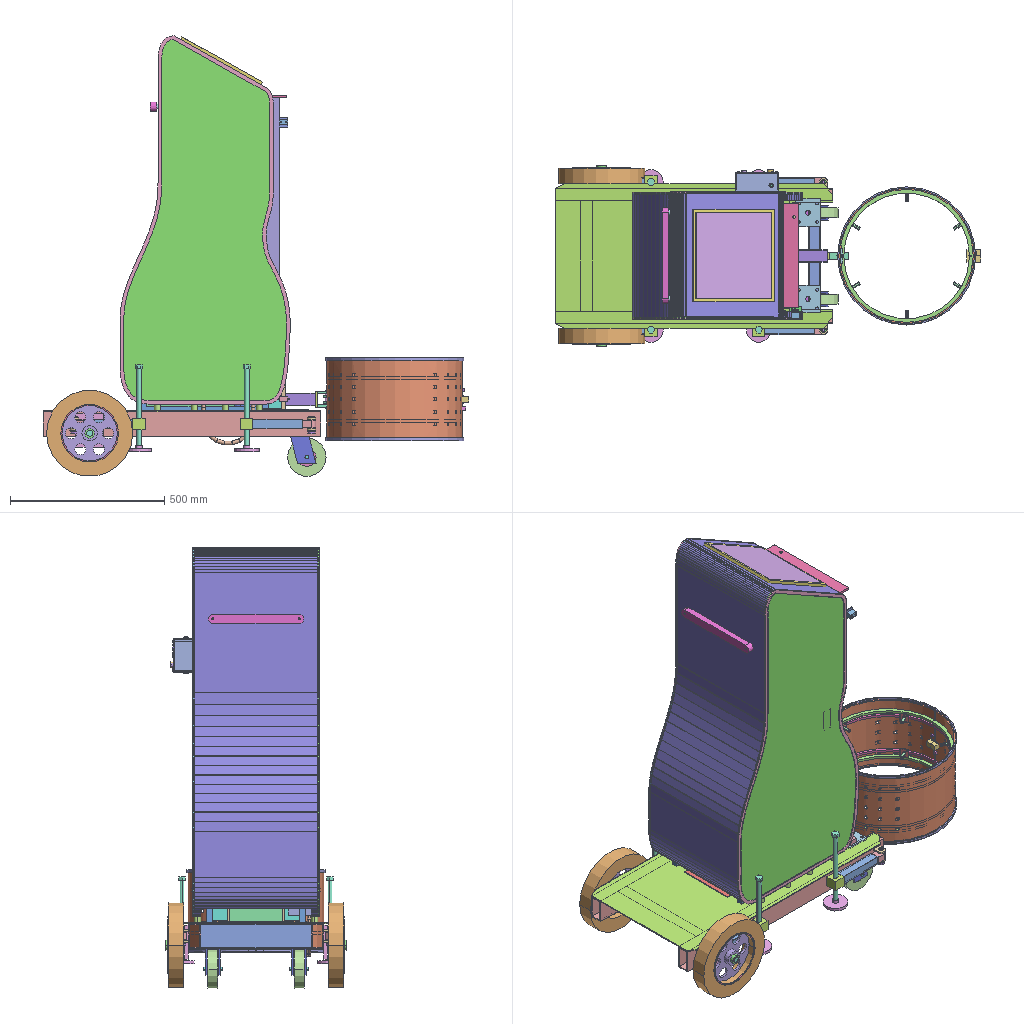Assembly | SolidWorks | 128 different items | 321 placed | box 1380 x 590 x 1429 mm
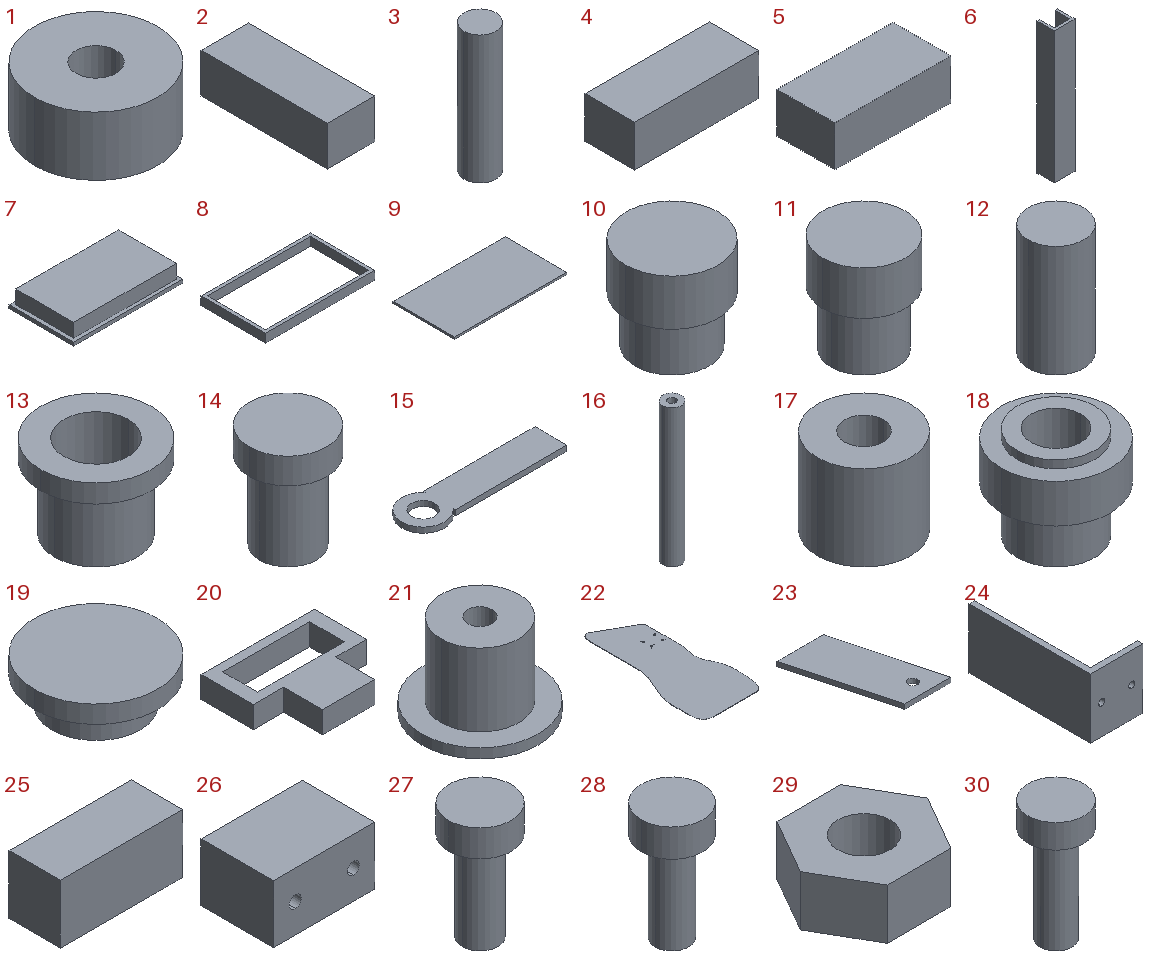Parts list (item | quantity | size | volume | features):
1 | x2 | 50 x 50 x 24 mm | 42177 mm3 | features Extrusion 1
2 | x1 | 12 x 32 x 10 mm | 3840 mm3 | features Extrusion 1
3 | x1 | 6 x 6 x 24 mm | 678.584 mm3 | features Extrusion 1
4 | x1 | 30 x 12 x 10 mm | 3600 mm3 | features Extrusion 1
5 | x1 | 20 x 10 x 7 mm | 1400 mm3 | features Extrusion 1
6 | x1 | 12 x 10 x 76 mm | 3306 mm3 | features Extrusion 1, ICE 1
7 | x1 | 64 x 38 x 10 mm | 21184 mm3 | features Extrusion 1, ICE 1
8 | x1 | 64 x 38 x 5 mm | 1771 mm3 | features Extrusion 1
9 | x1 | 58 x 32 x 1 mm | 1856 mm3 | features Extrusion 1
10 | x1 | 20 x 20 x 20 mm | 5152 mm3 | features Extrusion 1, ICE 1
11 | x1 | 15 x 15 x 18 mm | 2545 mm3 | features Extrusion 1, ICE 1
12 | x2 | 16 x 16 x 32 mm | 6434 mm3 | features Extrusion 1
13 | x1 | 12 x 12 x 9 mm | 325.155 mm3 | features Extrusion 1, ICE 1
14 | x1 | 6 x 6 x 8 mm | 147.781 mm3 | features Extrusion 1, ICE 1
15 | x1 | 28 x 8 x 1 mm | 158.117 mm3 | features Extrusion 1, ICE 1
16 | x4 | 8 x 8 x 60 mm | 2503 mm3 | features Extrusion 1
17 | x4 | 6 x 6 x 5.5 mm | 128.511 mm3 | features Extrusion 1
18 | x1 | 14 x 14 x 12 mm | 933.43 mm3 | features Extrusion 1, ICE 1
19 | x1 | 14 x 14 x 5 mm | 543.496 mm3 | features Extrusion 1, ICE 1
20 | x1 | 26 x 21 x 5 mm | 1300 mm3 | features Extrusion 1, ICE 1
21 | x4 | 12 x 12 x 8.5 mm | 448.364 mm3 | features Extrusion 1, ICE 1
22 | x1 | 552.5 x 1195 x 3 mm | 1469093 mm3 | features ICE 2, Extrusion 1
23 | x4 | 95 x 131 x 6 mm | 46459 mm3 | features Extrusion 1, ICE 1
24 | x1 | 28 x 65 x 32 mm | 8589 mm3 | features Extrusion 1, ICE 1
25 | x4 | 25 x 10.5 x 12 mm | 3150 mm3 | features Extrusion 1
26 | x1 | 28 x 20 x 16 mm | 8618 mm3 | features Extrusion 1, ICE 1
27 | x8 | 7 x 7 x 13 mm | 241.117 mm3 | features Extrusion 1, ICE 1
28 | x8 | 5.5 x 5.5 x 10.5 mm | 115.944 mm3 | features Extrusion 1, ICE 1
29 | x1 | 8.083 x 7 x 3.2 mm | 108.423 mm3 | features Extrusion 1
30 | x1 | 7 x 7 x 15 mm | 266.25 mm3 | features Extrusion 1, ICE 1
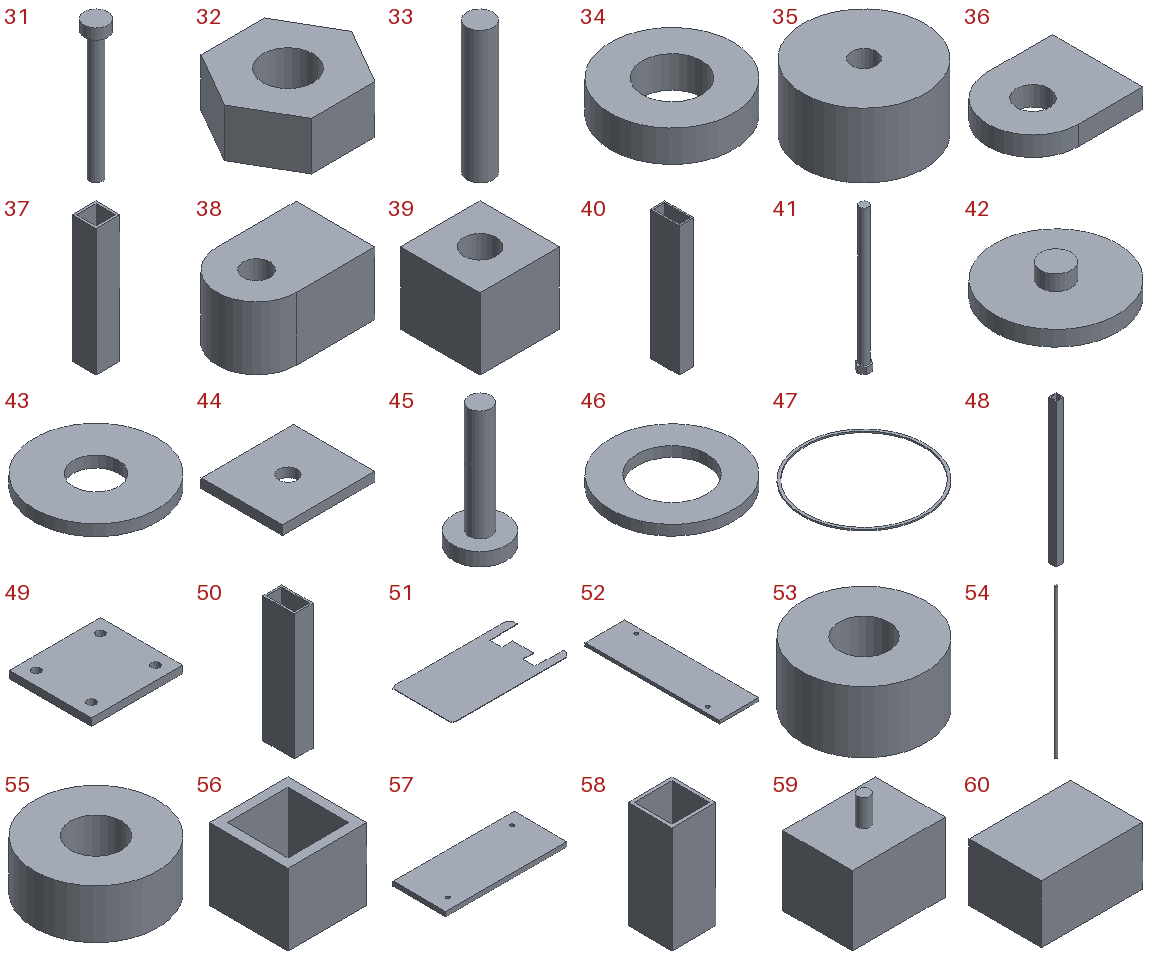31 | x2 | 5.5 x 5.5 x 32.5 mm | 271.453 mm3 | features Extrusion 1, ICE 1
32 | x2 | 6.351 x 5.5 x 2.4 mm | 51.092 mm3 | features Extrusion 1
33 | x2 | 12 x 12 x 60 mm | 6786 mm3 | features Extrusion 1
34 | x2 | 125 x 125 x 32 mm | 302221 mm3 | features Extrusion 1
35 | x2 | 60 x 60 x 32 mm | 86737 mm3 | features Extrusion 1
36 | x8 | 34 x 28 x 6 mm | 4717 mm3 | features Extrusion 1
37 | x4 | 30 x 30 x 160 mm | 51840 mm3 | features Extrusion 1
38 | x4 | 45 x 30 x 24 mm | 28121 mm3 | features Extrusion 1
39 | x4 | 40 x 40 x 36 mm | 49995 mm3 | features Extrusion 1, ICE 1
40 | x4 | 40 x 80 x 360 mm | 322560 mm3 | features Extrusion 1
41 | x4 | 24 x 20.785 x 262 mm | 54755 mm3 | features Extrusion 1, ICE 1
42 | x4 | 80 x 80 x 20 mm | 53407 mm3 | features Extrusion 1, ICE 1
43 | x2 | 44 x 44 x 4 mm | 5258 mm3 | features Extrusion 1
44 | x2 | 80 x 70 x 8 mm | 43151 mm3 | features Extrusion 1, ICE 1
45 | x4 | 24 x 24 x 56 mm | 6641 mm3 | features Extrusion 1, ICE 1
46 | x8 | 18 x 18 x 1.5 mm | 259.134 mm3 | features Extrusion 1
47 | x2 | 188 x 188 x 2 mm | 4624 mm3 | features Extrusion 1
48 | x2 | 50 x 50 x 1012 mm | 744832 mm3 | features Extrusion 1
49 | x2 | 100 x 90 x 8 mm | 69964 mm3 | features Extrusion 1, ICE 1
50 | x1 | 30 x 50 x 200 mm | 88800 mm3 | features Extrusion 1
51 | x1 | 900 x 470 x 3 mm | 1083288 mm3 | features Extrusion 1, ICE 1
52 | x1 | 100 x 340 x 8 mm | 270982 mm3 | features Extrusion 1, ICE 1
53 | x1 | 40 x 40 x 20 mm | 21010 mm3 | features Extrusion 1
54 | x1 | 16 x 16 x 970 mm | 195030 mm3 | features Extrusion 1
55 | x1 | 40 x 40 x 16 mm | 16726 mm3 | features Extrusion 1
56 | x2 | 66 x 66 x 60 mm | 105300 mm3 | features Extrusion 1
57 | x1 | 320 x 140 x 12 mm | 536073 mm3 | features Extrusion 1, ICE 1
58 | x1 | 40 x 40 x 97 mm | 43068 mm3 | features Extrusion 1
59 | x1 | 120 x 90 x 160 mm | 986074 mm3 | features Extrusion 1, ICE 1
60 | x1 | 28 x 20 x 16 mm | 8960 mm3 | features Extrusion 1
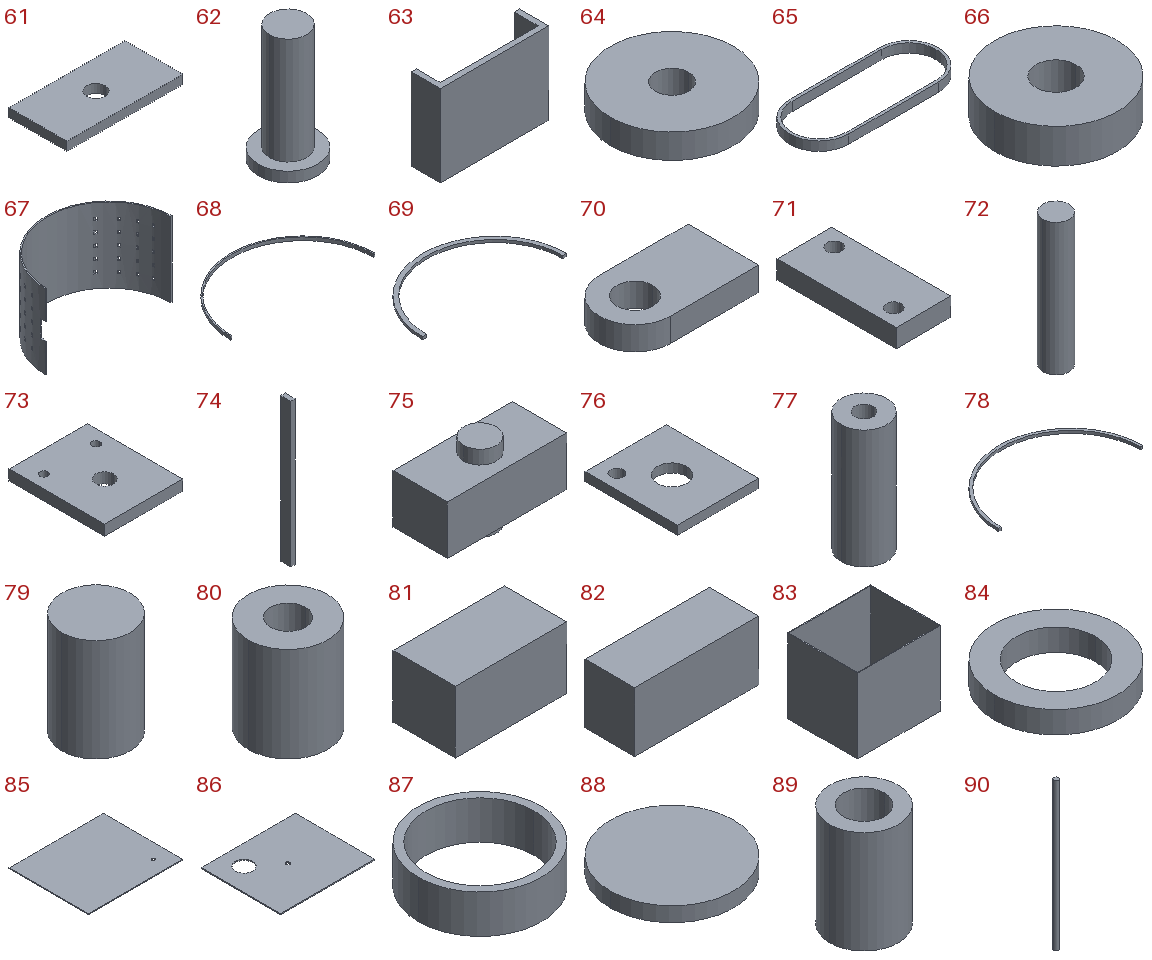61 | x1 | 40 x 20 x 3 mm | 2303 mm3 | features Extrusion 1, ICE 1
62 | x2 | 32 x 32 x 63 mm | 22488 mm3 | features Extrusion 1, ICE 1
63 | x1 | 120 x 32 x 90 mm | 92880 mm3 | features Extrusion 1
64 | x2 | 60 x 60 x 12 mm | 31456 mm3 | features Extrusion 1
65 | x1 | 166 x 66 x 10 mm | 11938 mm3 | features Extrusion 1
66 | x1 | 50 x 50 x 14 mm | 24603 mm3 | features Extrusion 1
67 | x2 | 439.995 x 219 x 260 mm | 692901 mm3 | features ICE 2, Extrusion 1
68 | x4 | 447.996 x 223 x 10 mm | 26438 mm3 | features Extrusion 1
69 | x4 | 431.995 x 215 x 8 mm | 63143 mm3 | features Extrusion 1
70 | x4 | 42 x 24 x 8 mm | 6634 mm3 | features Extrusion 1
71 | x1 | 24 x 52 x 8 mm | 9469 mm3 | features Extrusion 1, ICE 1
72 | x1 | 12 x 12 x 60 mm | 6786 mm3 | features Extrusion 1
73 | x2 | 90 x 110 x 12 mm | 113427 mm3 | features Extrusion 1, ICE 1
74 | x2 | 8 x 18 x 260 mm | 37440 mm3 | features Extrusion 1
75 | x2 | 44 x 20 x 28 mm | 16971 mm3 | features Extrusion 1, ICE 1
76 | x12 | 28 x 32 x 3 mm | 2397 mm3 | features Extrusion 1, ICE 1
77 | x12 | 10 x 10 x 26 mm | 1715 mm3 | features Extrusion 1
78 | x4 | 437.995 x 218 x 8 mm | 43100 mm3 | features Extrusion 1
79 | x12 | 8 x 8 x 12 mm | 603.186 mm3 | features Extrusion 1
80 | x12 | 10 x 10 x 12 mm | 760.014 mm3 | features Extrusion 1
81 | x1 | 18 x 10 x 10 mm | 1800 mm3 | features Extrusion 1
82 | x1 | 25 x 10 x 12 mm | 3000 mm3 | features Extrusion 1
83 | x1 | 380 x 320 x 340 mm | 1415760 mm3 | features Extrusion 1
84 | x2 | 280 x 280 x 50 mm | 1806416 mm3 | features Extrusion 1
85 | x1 | 380 x 320 x 3 mm | 364461 mm3 | features Extrusion 1, ICE 1
86 | x1 | 386 x 326 x 4 mm | 487146 mm3 | features Extrusion 1, ICE 1
87 | x2 | 80 x 80 x 25 mm | 29452 mm3 | features Extrusion 1
88 | x2 | 84 x 84 x 10 mm | 55418 mm3 | features Extrusion 1
89 | x1 | 20 x 20 x 30 mm | 6032 mm3 | features Extrusion 1
90 | x1 | 12 x 12 x 380 mm | 42977 mm3 | features Extrusion 1
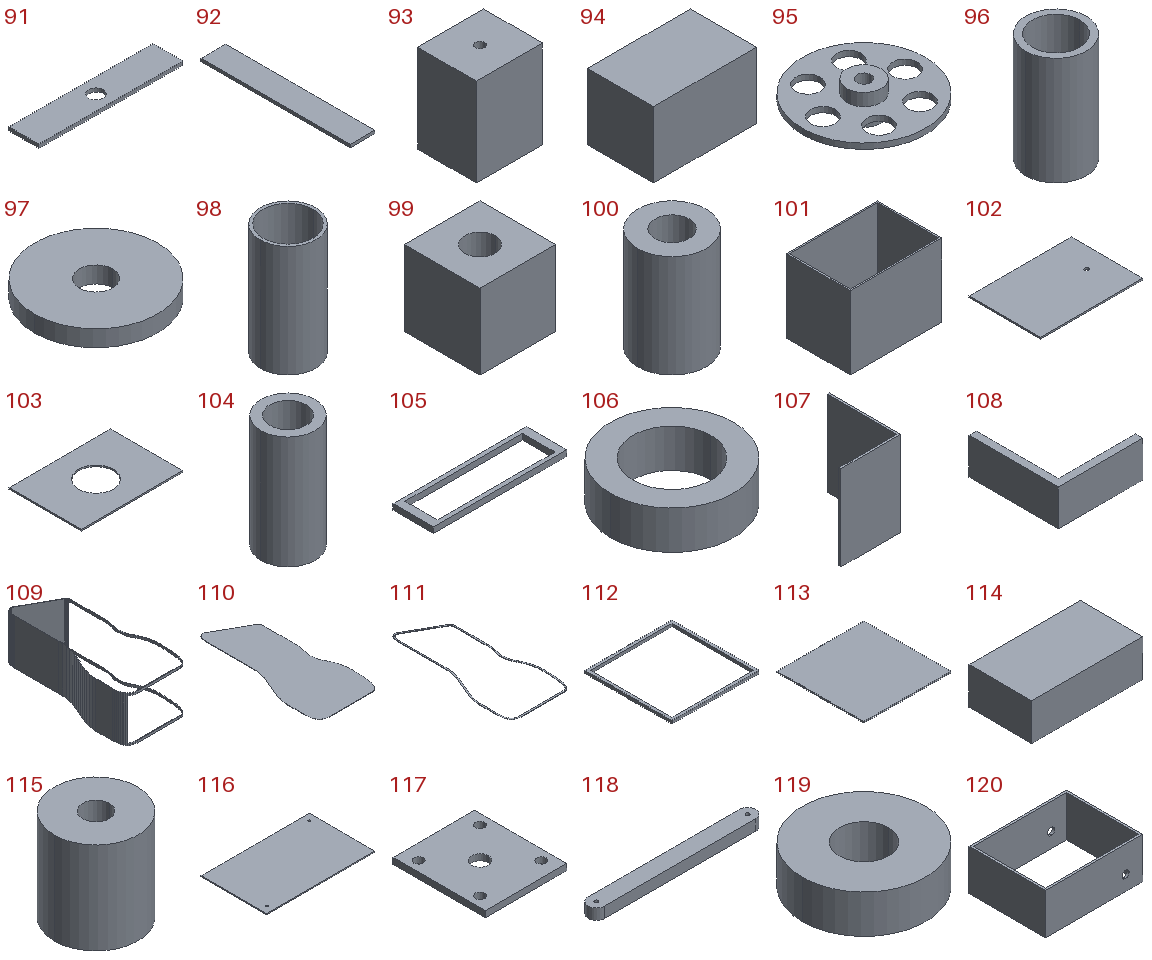91 | x1 | 120 x 25 x 3 mm | 8649 mm3 | features Extrusion 1, ICE 1
92 | x2 | 25 x 150 x 3 mm | 11250 mm3 | features Extrusion 1
93 | x1 | 90 x 80 x 120 mm | 849508 mm3 | features Extrusion 1, ICE 1
94 | x1 | 140 x 90 x 90 mm | 1134000 mm3 | features Extrusion 1
95 | x2 | 180 x 180 x 44 mm | 211302 mm3 | features ICE 2, Extrusion 1
96 | x1 | 56 x 56 x 100 mm | 94248 mm3 | features Extrusion 1
97 | x2 | 60 x 60 x 8 mm | 20971 mm3 | features Extrusion 1
98 | x1 | 40 x 40 x 80 mm | 19101 mm3 | features Extrusion 1
99 | x1 | 40 x 40 x 40 mm | 55755 mm3 | features Extrusion 1, ICE 1
100 | x7 | 16 x 16 x 24 mm | 3619 mm3 | features Extrusion 1
101 | x1 | 200 x 140 x 160 mm | 320640 mm3 | features Extrusion 1
102 | x1 | 200 x 140 x 3 mm | 83849 mm3 | features Extrusion 1, ICE 1
103 | x1 | 206 x 146 x 3 mm | 78683 mm3 | features Extrusion 1, ICE 1
104 | x32 | 12 x 12 x 25 mm | 1571 mm3 | features Extrusion 1
105 | x2 | 420 x 127 x 18 mm | 280800 mm3 | features Extrusion 1
106 | x2 | 32 x 32 x 10 mm | 4838 mm3 | features Extrusion 1
107 | x1 | 155 x 185 x 220 mm | 368500 mm3 | features Extrusion 1
108 | x1 | 70 x 74 x 30 mm | 24840 mm3 | features Extrusion 1
109 | x1 | 552.5 x 1195 x 400 mm | 2091406 mm3 | features ICE 2, Extrusion 1
110 | x1 | 552.5 x 1195 x 3 mm | 1470925 mm3 | features Extrusion 1, ICE 1
111 | x2 | 552.5 x 1195 x 3 mm | 110448 mm3 | features Extrusion 1
112 | x1 | 300 x 300 x 10 mm | 116000 mm3 | features Extrusion 1
113 | x1 | 280 x 280 x 4 mm | 313600 mm3 | features Extrusion 1
114 | x1 | 300 x 170 x 100 mm | 5100000 mm3 | features Extrusion 1
115 | x6 | 20 x 20 x 22 mm | 6204 mm3 | features Extrusion 1
116 | x1 | 330 x 200 x 3 mm | 197807 mm3 | features Extrusion 1, ICE 1
117 | x2 | 80 x 90 x 6 mm | 40436 mm3 | features Extrusion 1, ICE 1
118 | x1 | 310 x 30 x 20 mm | 180850 mm3 | features Extrusion 1, ICE 1
119 | x2 | 16 x 16 x 5 mm | 844.46 mm3 | features Extrusion 1
120 | x1 | 140 x 110 x 59 mm | 85886 mm3 | features Extrusion 1, ICE 1
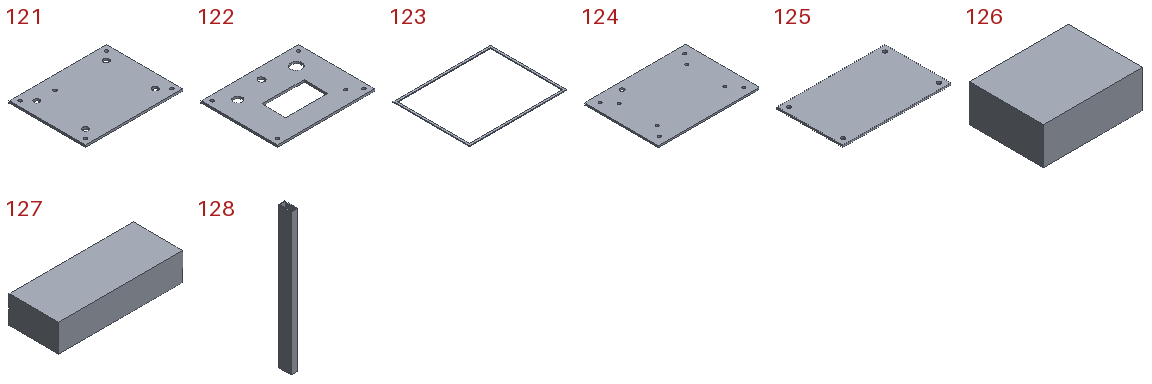121 | x1 | 140 x 110 x 3 mm | 45343 mm3 | features Extrusion 1
122 | x1 | 140 x 110 x 3 mm | 38560 mm3 | features Extrusion 1
123 | x1 | 140 x 110 x 1 mm | 1464 mm3 | features Extrusion 1
124 | x1 | 120 x 88 x 2 mm | 20938 mm3 | features Extrusion 1, ICE 1
125 | x1 | 90 x 55 x 1.6 mm | 7865 mm3 | features Extrusion 1
126 | x1 | 32 x 24 x 12 mm | 9216 mm3 | features Extrusion 1
127 | x1 | 45 x 18 x 10 mm | 8100 mm3 | features Extrusion 1
128 | x2 | 40 x 80 x 900 mm | 806400 mm3 | features Extrusion 1
Mates (type | each side: item.copy, entity, surface, feature):
Lock | 22.1 select_type:0 | 121.1 select_type:0
Lock | 120.1 select_type:0 | 121.1 select_type:0
Lock | 121.1 select_type:0 | 15.1 select_type:0
Lock | 120.1 select_type:0 | 18.1 select_type:0
Lock | 120.1 select_type:0 | 19.1 select_type:0
Lock | 22.1 select_type:0 | 30.1 select_type:0
Lock | 15.1 select_type:0 | 29.1 select_type:0
Lock | 48.1 select_type:0 | 24.1 select_type:0
Lock | 26.1 select_type:0 | 24.1 select_type:0
Lock | 121.1 select_type:0 | 16.1 select_type:0
Lock | 22.1 select_type:0 | 27.1 select_type:0
Lock | 121.1 select_type:0 | 16.2 select_type:0
Lock | 22.1 select_type:0 | 27.2 select_type:0
Lock | 121.1 select_type:0 | 16.3 select_type:0
Lock | 22.1 select_type:0 | 27.3 select_type:0
Lock | 121.1 select_type:0 | 16.4 select_type:0
Lock | 22.1 select_type:0 | 27.4 select_type:0
Lock | 121.1 select_type:0 | 21.1 select_type:0
Lock | 121.1 select_type:0 | 21.2 select_type:0
Lock | 121.1 select_type:0 | 21.3 select_type:0
Lock | 121.1 select_type:0 | 21.4 select_type:0
Lock | 26.1 select_type:0 | 31.1 select_type:0
Lock | 26.1 select_type:0 | 31.2 select_type:0
Lock | 24.1 select_type:0 | 32.1 select_type:0
Lock | 83.1 select_type:0 | 25.1 select_type:0
Lock | 83.1 select_type:0 | 25.2 select_type:0
Lock | 83.1 select_type:0 | 25.3 select_type:0
Lock | 83.1 select_type:0 | 25.4 select_type:0
Lock | 122.1 select_type:0 | 16.1 select_type:0
Lock | 122.1 select_type:0 | 123.1 select_type:0
Lock | 124.1 select_type:0 | 21.1 select_type:0
Lock | 124.1 select_type:0 | 6.1 select_type:0
Lock | 122.1 select_type:0 | 8.1 select_type:0
Lock | 122.1 select_type:0 | 10.1 select_type:0
Lock | 122.1 select_type:0 | 11.1 select_type:0
Lock | 122.1 select_type:0 | 13.1 select_type:0
Lock | 122.1 select_type:0 | 14.1 select_type:0
Lock | 124.1 select_type:0 | 20.1 select_type:0
Lock | 122.1 select_type:0 | 27.5 select_type:0
Lock | 122.1 select_type:0 | 27.6 select_type:0
Lock | 122.1 select_type:0 | 27.7 select_type:0
Lock | 122.1 select_type:0 | 27.8 select_type:0
Lock | 124.1 select_type:0 | 17.1 select_type:0
Lock | 124.1 select_type:0 | 17.2 select_type:0
Lock | 124.1 select_type:0 | 17.3 select_type:0
Lock | 124.1 select_type:0 | 17.4 select_type:0
Lock | 124.1 select_type:0 | 28.1 select_type:0
Lock | 124.1 select_type:0 | 28.2 select_type:0
Lock | 124.1 select_type:0 | 28.3 select_type:0
Lock | 124.1 select_type:0 | 28.4 select_type:0
Lock | 125.1 select_type:0 | 17.1 select_type:0
Lock | 125.1 select_type:0 | 126.1 select_type:0
Lock | 125.1 select_type:0 | 127.1 select_type:0
Lock | 125.1 select_type:0 | 2.1 select_type:0
Lock | 2.1 select_type:0 | 3.1 select_type:0
Lock | 4.1 select_type:0 | 6.1 select_type:0
Lock | 5.1 select_type:0 | 6.1 select_type:0
Lock | 7.1 select_type:0 | 8.1 select_type:0
Lock | 7.1 select_type:0 | 9.1 select_type:0
Lock | 125.1 select_type:0 | 28.5 select_type:0
Lock | 125.1 select_type:0 | 28.6 select_type:0
Lock | 125.1 select_type:0 | 28.7 select_type:0
Lock | 125.1 select_type:0 | 28.8 select_type:0
Lock | 92.1 select_type:0 | 25.1 select_type:0
Lock | 92.2 select_type:0 | 25.3 select_type:0
Lock | 24.1 select_type:0 | 32.2 select_type:0